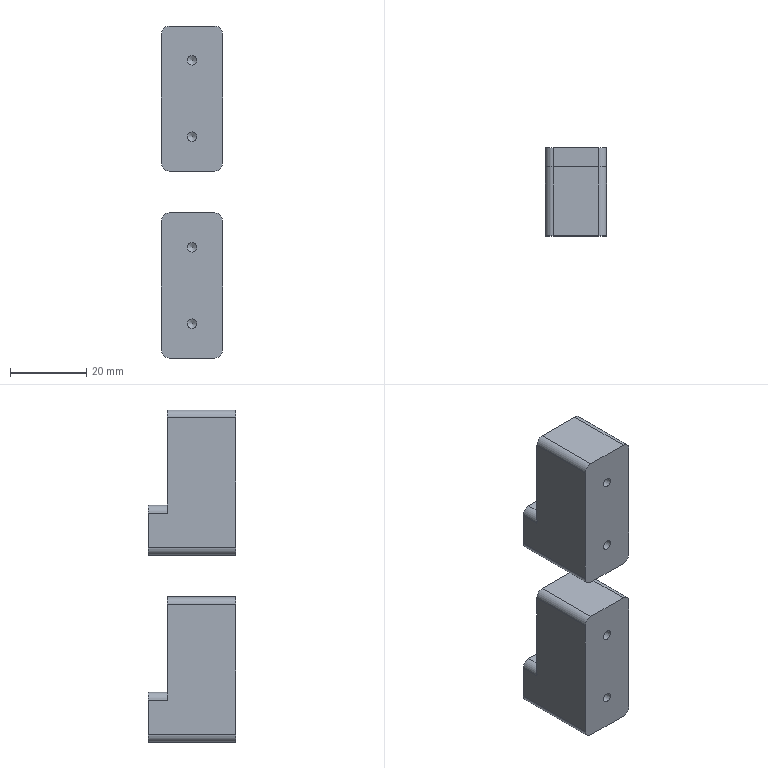Part | NX | 2 solids | 40 faces | box 16 x 23 x 87 mm | volume 23381 mm3 | cylinder 18 | plane 16 | cone 6 | commonest cylinder face diameters 4 x12 2.5 x4 3.3 x2
STEP:
#1=CARTESIAN_POINT('',(0.,18.,64.65));
#2=VERTEX_POINT('',#1);
#3=CARTESIAN_POINT('',(0.,18.,63.));
#4=DIRECTION('',(0.,1.,0.));
#5=DIRECTION('',(0.,0.,1.));
#6=AXIS2_PLACEMENT_3D('',#3,#4,#5);
#7=CIRCLE('',#6,1.65);
#8=EDGE_CURVE('',#2,#2,#7,.T.);
#9=ORIENTED_EDGE('',*,*,#8,.T.);
#10=EDGE_LOOP('',(#9));
#11=FACE_BOUND('',#10,.T.);
#12=CARTESIAN_POINT('',(0.,7.9,64.65));
#13=VERTEX_POINT('',#12);
#14=CARTESIAN_POINT('',(0.,7.9,63.));
#15=DIRECTION('',(0.,1.,0.));
#16=DIRECTION('',(0.,0.,1.));
#17=AXIS2_PLACEMENT_3D('',#14,#15,#16);
#18=CIRCLE('',#17,1.65);
#19=EDGE_CURVE('',#13,#13,#18,.T.);
#20=ORIENTED_EDGE('',*,*,#19,.F.);
#21=EDGE_LOOP('',(#20));
#22=FACE_BOUND('',#21,.T.);
#23=CARTESIAN_POINT('',(0.,18.,63.));
#24=DIRECTION('',(0.,1.,0.));
#25=DIRECTION('',(0.,0.,1.));
#26=AXIS2_PLACEMENT_3D('',#23,#24,#25);
#27=CYLINDRICAL_SURFACE('',#26,1.65);
#28=ADVANCED_FACE('',(#11,#22),#27,.F.);
#29=CARTESIAN_POINT('',(0.,6.909,63.));
#30=VERTEX_POINT('',#29);
#31=VERTEX_LOOP('',#30);
#32=FACE_BOUND('',#31,.T.);
#33=ORIENTED_EDGE('',*,*,#19,.T.);
#34=EDGE_LOOP('',(#33));
#35=FACE_BOUND('',#34,.T.);
#36=CARTESIAN_POINT('',(0.,7.9,63.));
#37=DIRECTION('',(0.,1.,0.));
#38=DIRECTION('',(0.,0.,1.));
#39=AXIS2_PLACEMENT_3D('',#36,#37,#38);
#40=CONICAL_SURFACE('',#39,1.65,1.03);
#41=ADVANCED_FACE('',(#32,#35),#40,.F.);
#42=CARTESIAN_POINT('',(6.,18.,68.));
#43=VERTEX_POINT('',#42);
#44=CARTESIAN_POINT('',(8.,18.,66.));
#45=VERTEX_POINT('',#44);
#46=CARTESIAN_POINT('',(6.,18.,66.));
#47=DIRECTION('',(0.,1.,0.));
#48=DIRECTION('',(0.,0.,-1.));
#49=AXIS2_PLACEMENT_3D('',#46,#47,#48);
#50=CIRCLE('',#49,2.);
#51=EDGE_CURVE('',#43,#45,#50,.T.);
#52=ORIENTED_EDGE('',*,*,#51,.F.);
#53=CARTESIAN_POINT('',(6.,0.,68.));
#54=VERTEX_POINT('',#53);
#55=CARTESIAN_POINT('',(6.,23.,68.));
#56=DIRECTION('',(0.,1.,0.));
#57=VECTOR('',#56,1000.);
#58=LINE('',#55,#57);
#59=EDGE_CURVE('',#54,#43,#58,.T.);
#60=ORIENTED_EDGE('',*,*,#59,.F.);
#61=CARTESIAN_POINT('',(8.,0.,66.));
#62=VERTEX_POINT('',#61);
#63=CARTESIAN_POINT('',(6.,0.,66.));
#64=DIRECTION('',(0.,-1.,0.));
#65=DIRECTION('',(0.,0.,-1.));
#66=AXIS2_PLACEMENT_3D('',#63,#64,#65);
#67=CIRCLE('',#66,2.);
#68=EDGE_CURVE('',#62,#54,#67,.T.);
#69=ORIENTED_EDGE('',*,*,#68,.F.);
#70=CARTESIAN_POINT('',(8.,23.,66.));
#71=DIRECTION('',(0.,-1.,0.));
#72=VECTOR('',#71,1000.);
#73=LINE('',#70,#72);
#74=EDGE_CURVE('',#45,#62,#73,.T.);
#75=ORIENTED_EDGE('',*,*,#74,.F.);
#76=EDGE_LOOP('',(#52,#60,#69,#75));
#77=FACE_BOUND('',#76,.T.);
#78=CARTESIAN_POINT('',(6.,23.,66.));
#79=DIRECTION('',(0.,-1.,0.));
#80=DIRECTION('',(0.,0.,-1.));
#81=AXIS2_PLACEMENT_3D('',#78,#79,#80);
#82=CYLINDRICAL_SURFACE('',#81,2.);
#83=ADVANCED_FACE('',(#77),#82,.T.);
#84=CARTESIAN_POINT('',(8.,23.,32.));
#85=VERTEX_POINT('',#84);
#86=CARTESIAN_POINT('',(6.,23.,30.));
#87=VERTEX_POINT('',#86);
#88=CARTESIAN_POINT('',(6.,23.,32.));
#89=DIRECTION('',(0.,1.,0.));
#90=DIRECTION('',(0.,0.,-1.));
#91=AXIS2_PLACEMENT_3D('',#88,#89,#90);
#92=CIRCLE('',#91,2.);
#93=EDGE_CURVE('',#85,#87,#92,.T.);
#94=ORIENTED_EDGE('',*,*,#93,.F.);
#95=CARTESIAN_POINT('',(8.,0.,32.));
#96=VERTEX_POINT('',#95);
#97=CARTESIAN_POINT('',(8.,23.,32.));
#98=DIRECTION('',(0.,1.,0.));
#99=VECTOR('',#98,1000.);
#100=LINE('',#97,#99);
#101=EDGE_CURVE('',#96,#85,#100,.T.);
#102=ORIENTED_EDGE('',*,*,#101,.F.);
#103=CARTESIAN_POINT('',(6.,0.,30.));
#104=VERTEX_POINT('',#103);
#105=CARTESIAN_POINT('',(6.,0.,32.));
#106=DIRECTION('',(0.,-1.,0.));
#107=DIRECTION('',(0.,0.,-1.));
#108=AXIS2_PLACEMENT_3D('',#105,#106,#107);
#109=CIRCLE('',#108,2.);
#110=EDGE_CURVE('',#104,#96,#109,.T.);
#111=ORIENTED_EDGE('',*,*,#110,.F.);
#112=CARTESIAN_POINT('',(6.,23.,30.));
#113=DIRECTION('',(0.,-1.,0.));
#114=VECTOR('',#113,1000.);
#115=LINE('',#112,#114);
#116=EDGE_CURVE('',#87,#104,#115,.T.);
#117=ORIENTED_EDGE('',*,*,#116,.F.);
#118=EDGE_LOOP('',(#94,#102,#111,#117));
#119=FACE_BOUND('',#118,.T.);
#120=CARTESIAN_POINT('',(6.,23.,32.));
#121=DIRECTION('',(0.,-1.,0.));
#122=DIRECTION('',(0.,0.,-1.));
#123=AXIS2_PLACEMENT_3D('',#120,#121,#122);
#124=CYLINDRICAL_SURFACE('',#123,2.);
#125=ADVANCED_FACE('',(#119),#124,.T.);
#126=CARTESIAN_POINT('',(-6.,23.,30.));
#127=VERTEX_POINT('',#126);
#128=CARTESIAN_POINT('',(-8.,23.,32.));
#129=VERTEX_POINT('',#128);
#130=CARTESIAN_POINT('',(-6.,23.,32.));
#131=DIRECTION('',(0.,1.,0.));
#132=DIRECTION('',(0.,0.,-1.));
#133=AXIS2_PLACEMENT_3D('',#130,#131,#132);
#134=CIRCLE('',#133,2.);
#135=EDGE_CURVE('',#127,#129,#134,.T.);
#136=ORIENTED_EDGE('',*,*,#135,.F.);
#137=CARTESIAN_POINT('',(-6.,0.,30.));
#138=VERTEX_POINT('',#137);
#139=CARTESIAN_POINT('',(-6.,23.,30.));
#140=DIRECTION('',(0.,1.,0.));
#141=VECTOR('',#140,1000.);
#142=LINE('',#139,#141);
#143=EDGE_CURVE('',#138,#127,#142,.T.);
#144=ORIENTED_EDGE('',*,*,#143,.F.);
#145=CARTESIAN_POINT('',(-8.,0.,32.));
#146=VERTEX_POINT('',#145);
#147=CARTESIAN_POINT('',(-6.,0.,32.));
#148=DIRECTION('',(0.,-1.,0.));
#149=DIRECTION('',(0.,0.,-1.));
#150=AXIS2_PLACEMENT_3D('',#147,#148,#149);
#151=CIRCLE('',#150,2.);
#152=EDGE_CURVE('',#146,#138,#151,.T.);
#153=ORIENTED_EDGE('',*,*,#152,.F.);
#154=CARTESIAN_POINT('',(-8.,23.,32.));
#155=DIRECTION('',(0.,-1.,0.));
#156=VECTOR('',#155,1000.);
#157=LINE('',#154,#156);
#158=EDGE_CURVE('',#129,#146,#157,.T.);
#159=ORIENTED_EDGE('',*,*,#158,.F.);
#160=EDGE_LOOP('',(#136,#144,#153,#159));
#161=FACE_BOUND('',#160,.T.);
#162=CARTESIAN_POINT('',(-6.,23.,32.));
#163=DIRECTION('',(0.,-1.,0.));
#164=DIRECTION('',(0.,0.,-1.));
#165=AXIS2_PLACEMENT_3D('',#162,#163,#164);
#166=CYLINDRICAL_SURFACE('',#165,2.);
#167=ADVANCED_FACE('',(#161),#166,.T.);
#168=CARTESIAN_POINT('',(-8.,18.,66.));
#169=VERTEX_POINT('',#168);
#170=CARTESIAN_POINT('',(-6.,18.,68.));
#171=VERTEX_POINT('',#170);
#172=CARTESIAN_POINT('',(-6.,18.,66.));
#173=DIRECTION('',(0.,1.,0.));
#174=DIRECTION('',(0.,0.,-1.));
#175=AXIS2_PLACEMENT_3D('',#172,#173,#174);
#176=CIRCLE('',#175,2.);
#177=EDGE_CURVE('',#169,#171,#176,.T.);
#178=ORIENTED_EDGE('',*,*,#177,.F.);
#179=CARTESIAN_POINT('',(-8.,0.,66.));
#180=VERTEX_POINT('',#179);
#181=CARTESIAN_POINT('',(-8.,23.,66.));
#182=DIRECTION('',(0.,1.,0.));
#183=VECTOR('',#182,1000.);
#184=LINE('',#181,#183);
#185=EDGE_CURVE('',#180,#169,#184,.T.);
#186=ORIENTED_EDGE('',*,*,#185,.F.);
#187=CARTESIAN_POINT('',(-6.,0.,68.));
#188=VERTEX_POINT('',#187);
#189=CARTESIAN_POINT('',(-6.,0.,66.));
#190=DIRECTION('',(0.,-1.,0.));
#191=DIRECTION('',(0.,0.,-1.));
#192=AXIS2_PLACEMENT_3D('',#189,#190,#191);
#193=CIRCLE('',#192,2.);
#194=EDGE_CURVE('',#188,#180,#193,.T.);
#195=ORIENTED_EDGE('',*,*,#194,.F.);
#196=CARTESIAN_POINT('',(-6.,23.,68.));
#197=DIRECTION('',(0.,-1.,0.));
#198=VECTOR('',#197,1000.);
#199=LINE('',#196,#198);
#200=EDGE_CURVE('',#171,#188,#199,.T.);
#201=ORIENTED_EDGE('',*,*,#200,.F.);
#202=EDGE_LOOP('',(#178,#186,#195,#201));
#203=FACE_BOUND('',#202,.T.);
#204=CARTESIAN_POINT('',(-6.,23.,66.));
#205=DIRECTION('',(0.,-1.,0.));
#206=DIRECTION('',(0.,0.,-1.));
#207=AXIS2_PLACEMENT_3D('',#204,#205,#206);
#208=CYLINDRICAL_SURFACE('',#207,2.);
#209=ADVANCED_FACE('',(#203),#208,.T.);
#210=CARTESIAN_POINT('',(-6.,18.,43.));
#211=VERTEX_POINT('',#210);
#212=CARTESIAN_POINT('',(-8.,18.,41.));
#213=VERTEX_POINT('',#212);
#214=CARTESIAN_POINT('',(-6.,18.,41.));
#215=DIRECTION('',(0.,-1.,0.));
#216=DIRECTION('',(0.,0.,-1.));
#217=AXIS2_PLACEMENT_3D('',#214,#215,#216);
#218=CIRCLE('',#217,2.);
#219=EDGE_CURVE('',#211,#213,#218,.T.);
#220=ORIENTED_EDGE('',*,*,#219,.F.);
#221=CARTESIAN_POINT('',(-6.,23.,43.));
#222=VERTEX_POINT('',#221);
#223=CARTESIAN_POINT('',(-6.,18.,43.));
#224=DIRECTION('',(0.,-1.,0.));
#225=VECTOR('',#224,1000.);
#226=LINE('',#223,#225);
#227=EDGE_CURVE('',#222,#211,#226,.T.);
#228=ORIENTED_EDGE('',*,*,#227,.F.);
#229=CARTESIAN_POINT('',(-8.,23.,41.));
#230=VERTEX_POINT('',#229);
#231=CARTESIAN_POINT('',(-6.,23.,41.));
#232=DIRECTION('',(0.,1.,0.));
#233=DIRECTION('',(0.,0.,-1.));
#234=AXIS2_PLACEMENT_3D('',#231,#232,#233);
#235=CIRCLE('',#234,2.);
#236=EDGE_CURVE('',#230,#222,#235,.T.);
#237=ORIENTED_EDGE('',*,*,#236,.F.);
#238=CARTESIAN_POINT('',(-8.,23.,41.));
#239=DIRECTION('',(0.,1.,0.));
#240=VECTOR('',#239,1000.);
#241=LINE('',#238,#240);
#242=EDGE_CURVE('',#213,#230,#241,.T.);
#243=ORIENTED_EDGE('',*,*,#242,.F.);
#244=EDGE_LOOP('',(#220,#228,#237,#243));
#245=FACE_BOUND('',#244,.T.);
#246=CARTESIAN_POINT('',(-6.,23.,41.));
#247=DIRECTION('',(0.,-1.,0.));
#248=DIRECTION('',(0.,0.,-1.));
#249=AXIS2_PLACEMENT_3D('',#246,#247,#248);
#250=CYLINDRICAL_SURFACE('',#249,2.);
#251=ADVANCED_FACE('',(#245),#250,.T.);
#252=CARTESIAN_POINT('',(8.,18.,41.));
#253=VERTEX_POINT('',#252);
#254=CARTESIAN_POINT('',(6.,18.,43.));
#255=VERTEX_POINT('',#254);
#256=CARTESIAN_POINT('',(6.,18.,41.));
#257=DIRECTION('',(0.,-1.,0.));
#258=DIRECTION('',(0.,0.,-1.));
#259=AXIS2_PLACEMENT_3D('',#256,#257,#258);
#260=CIRCLE('',#259,2.);
#261=EDGE_CURVE('',#253,#255,#260,.T.);
#262=ORIENTED_EDGE('',*,*,#261,.F.);
#263=CARTESIAN_POINT('',(8.,23.,41.));
#264=VERTEX_POINT('',#263);
#265=CARTESIAN_POINT('',(8.,18.,41.));
#266=DIRECTION('',(0.,-1.,0.));
#267=VECTOR('',#266,1000.);
#268=LINE('',#265,#267);
#269=EDGE_CURVE('',#264,#253,#268,.T.);
#270=ORIENTED_EDGE('',*,*,#269,.F.);
#271=CARTESIAN_POINT('',(6.,23.,43.));
#272=VERTEX_POINT('',#271);
#273=CARTESIAN_POINT('',(6.,23.,41.));
#274=DIRECTION('',(0.,1.,0.));
#275=DIRECTION('',(0.,0.,-1.));
#276=AXIS2_PLACEMENT_3D('',#273,#274,#275);
#277=CIRCLE('',#276,2.);
#278=EDGE_CURVE('',#272,#264,#277,.T.);
#279=ORIENTED_EDGE('',*,*,#278,.F.);
#280=CARTESIAN_POINT('',(6.,23.,43.));
#281=DIRECTION('',(0.,1.,0.));
#282=VECTOR('',#281,1000.);
#283=LINE('',#280,#282);
#284=EDGE_CURVE('',#255,#272,#283,.T.);
#285=ORIENTED_EDGE('',*,*,#284,.F.);
#286=EDGE_LOOP('',(#262,#270,#279,#285));
#287=FACE_BOUND('',#286,.T.);
#288=CARTESIAN_POINT('',(6.,18.,41.));
#289=DIRECTION('',(0.,-1.,0.));
#290=DIRECTION('',(0.,0.,-1.));
#291=AXIS2_PLACEMENT_3D('',#288,#289,#290);
#292=CYLINDRICAL_SURFACE('',#291,2.);
#293=ADVANCED_FACE('',(#287),#292,.T.);
#294=CARTESIAN_POINT('',(-8.,18.,43.));
#295=DIRECTION('',(0.,0.,-1.));
#296=VECTOR('',#295,1000.);
#297=LINE('',#294,#296);
#298=EDGE_CURVE('',#169,#213,#297,.T.);
#299=ORIENTED_EDGE('',*,*,#298,.F.);
#300=ORIENTED_EDGE('',*,*,#177,.T.);
#301=CARTESIAN_POINT('',(8.,18.,68.));
#302=DIRECTION('',(-1.,0.,0.));
#303=VECTOR('',#302,1000.);
#304=LINE('',#301,#303);
#305=EDGE_CURVE('',#43,#171,#304,.T.);
#306=ORIENTED_EDGE('',*,*,#305,.F.);
#307=ORIENTED_EDGE('',*,*,#51,.T.);
#308=CARTESIAN_POINT('',(8.,18.,43.));
#309=DIRECTION('',(0.,0.,1.));
#310=VECTOR('',#309,1000.);
#311=LINE('',#308,#310);
#312=EDGE_CURVE('',#253,#45,#311,.T.);
#313=ORIENTED_EDGE('',*,*,#312,.F.);
#314=ORIENTED_EDGE('',*,*,#261,.T.);
#315=CARTESIAN_POINT('',(8.,18.,43.));
#316=DIRECTION('',(1.,0.,0.));
#317=VECTOR('',#316,1000.);
#318=LINE('',#315,#317);
#319=EDGE_CURVE('',#211,#255,#318,.T.);
#320=ORIENTED_EDGE('',*,*,#319,.F.);
#321=ORIENTED_EDGE('',*,*,#219,.T.);
#322=EDGE_LOOP('',(#299,#300,#306,#307,#313,#314,#320,#321));
#323=FACE_BOUND('',#322,.T.);
#324=ORIENTED_EDGE('',*,*,#8,.F.);
#325=EDGE_LOOP('',(#324));
#326=FACE_BOUND('',#325,.T.);
#327=CARTESIAN_POINT('',(0.,18.,49.));
#328=DIRECTION('',(0.,-1.,0.));
#329=DIRECTION('',(0.,0.,-1.));
#330=AXIS2_PLACEMENT_3D('',#327,#328,#329);
#331=PLANE('',#330);
#332=ADVANCED_FACE('',(#323,#326),#331,.F.);
#333=ORIENTED_EDGE('',*,*,#319,.T.);
#334=ORIENTED_EDGE('',*,*,#284,.T.);
#335=CARTESIAN_POINT('',(8.,23.,43.));
#336=DIRECTION('',(1.,0.,0.));
#337=VECTOR('',#336,1000.);
#338=LINE('',#335,#337);
#339=EDGE_CURVE('',#222,#272,#338,.T.);
#340=ORIENTED_EDGE('',*,*,#339,.F.);
#341=ORIENTED_EDGE('',*,*,#227,.T.);
#342=EDGE_LOOP('',(#333,#334,#340,#341));
#343=FACE_BOUND('',#342,.T.);
#344=CARTESIAN_POINT('',(8.,18.,43.));
#345=DIRECTION('',(0.,0.,1.));
#346=DIRECTION('',(1.,0.,0.));
#347=AXIS2_PLACEMENT_3D('',#344,#345,#346);
#348=PLANE('',#347);
#349=ADVANCED_FACE('',(#343),#348,.T.);
#350=CARTESIAN_POINT('',(0.,0.,37.75));
#351=VERTEX_POINT('',#350);
#352=CARTESIAN_POINT('',(0.,0.,39.));
#353=DIRECTION('',(0.,-1.,0.));
#354=DIRECTION('',(0.,0.,-1.));
#355=AXIS2_PLACEMENT_3D('',#352,#353,#354);
#356=CIRCLE('',#355,1.25);
#357=EDGE_CURVE('',#351,#351,#356,.T.);
#358=ORIENTED_EDGE('',*,*,#357,.T.);
#359=EDGE_LOOP('',(#358));
#360=FACE_BOUND('',#359,.T.);
#361=CARTESIAN_POINT('',(0.,12.5,37.75));
#362=VERTEX_POINT('',#361);
#363=CARTESIAN_POINT('',(0.,12.5,39.));
#364=DIRECTION('',(0.,-1.,0.));
#365=DIRECTION('',(0.,0.,-1.));
#366=AXIS2_PLACEMENT_3D('',#363,#364,#365);
#367=CIRCLE('',#366,1.25);
#368=EDGE_CURVE('',#362,#362,#367,.T.);
#369=ORIENTED_EDGE('',*,*,#368,.F.);
#370=EDGE_LOOP('',(#369));
#371=FACE_BOUND('',#370,.T.);
#372=CARTESIAN_POINT('',(0.,0.,39.));
#373=DIRECTION('',(0.,-1.,0.));
#374=DIRECTION('',(0.,0.,-1.));
#375=AXIS2_PLACEMENT_3D('',#372,#373,#374);
#376=CYLINDRICAL_SURFACE('',#375,1.25);
#377=ADVANCED_FACE('',(#360,#371),#376,.F.);
#378=CARTESIAN_POINT('',(0.,13.251,39.));
#379=VERTEX_POINT('',#378);
#380=VERTEX_LOOP('',#379);
#381=FACE_BOUND('',#380,.T.);
#382=ORIENTED_EDGE('',*,*,#368,.T.);
#383=EDGE_LOOP('',(#382));
#384=FACE_BOUND('',#383,.T.);
#385=CARTESIAN_POINT('',(0.,12.5,39.));
#386=DIRECTION('',(0.,-1.,0.));
#387=DIRECTION('',(0.,0.,-1.));
#388=AXIS2_PLACEMENT_3D('',#385,#386,#387);
#389=CONICAL_SURFACE('',#388,1.25,1.03);
#390=ADVANCED_FACE('',(#381,#384),#389,.F.);
#391=CARTESIAN_POINT('',(0.,0.,57.75));
#392=VERTEX_POINT('',#391);
#393=CARTESIAN_POINT('',(0.,0.,59.));
#394=DIRECTION('',(0.,-1.,0.));
#395=DIRECTION('',(0.,0.,-1.));
#396=AXIS2_PLACEMENT_3D('',#393,#394,#395);
#397=CIRCLE('',#396,1.25);
#398=EDGE_CURVE('',#392,#392,#397,.T.);
#399=ORIENTED_EDGE('',*,*,#398,.T.);
#400=EDGE_LOOP('',(#399));
#401=FACE_BOUND('',#400,.T.);
#402=CARTESIAN_POINT('',(0.,12.5,57.75));
#403=VERTEX_POINT('',#402);
#404=CARTESIAN_POINT('',(0.,12.5,59.));
#405=DIRECTION('',(0.,-1.,0.));
#406=DIRECTION('',(0.,0.,-1.));
#407=AXIS2_PLACEMENT_3D('',#404,#405,#406);
#408=CIRCLE('',#407,1.25);
#409=EDGE_CURVE('',#403,#403,#408,.T.);
#410=ORIENTED_EDGE('',*,*,#409,.F.);
#411=EDGE_LOOP('',(#410));
#412=FACE_BOUND('',#411,.T.);
#413=CARTESIAN_POINT('',(0.,0.,59.));
#414=DIRECTION('',(0.,-1.,0.));
#415=DIRECTION('',(0.,0.,-1.));
#416=AXIS2_PLACEMENT_3D('',#413,#414,#415);
#417=CYLINDRICAL_SURFACE('',#416,1.25);
#418=ADVANCED_FACE('',(#401,#412),#417,.F.);
#419=CARTESIAN_POINT('',(0.,13.251,59.));
#420=VERTEX_POINT('',#419);
#421=VERTEX_LOOP('',#420);
#422=FACE_BOUND('',#421,.T.);
#423=ORIENTED_EDGE('',*,*,#409,.T.);
#424=EDGE_LOOP('',(#423));
#425=FACE_BOUND('',#424,.T.);
#426=CARTESIAN_POINT('',(0.,12.5,59.));
#427=DIRECTION('',(0.,-1.,0.));
#428=DIRECTION('',(0.,0.,-1.));
#429=AXIS2_PLACEMENT_3D('',#426,#427,#428);
#430=CONICAL_SURFACE('',#429,1.25,1.03);
#431=ADVANCED_FACE('',(#422,#425),#430,.F.);
#432=CARTESIAN_POINT('',(-8.,0.,68.));
#433=DIRECTION('',(1.,0.,0.));
#434=VECTOR('',#433,1000.);
#435=LINE('',#432,#434);
#436=EDGE_CURVE('',#188,#54,#435,.T.);
#437=ORIENTED_EDGE('',*,*,#436,.F.);
#438=ORIENTED_EDGE('',*,*,#194,.T.);
#439=CARTESIAN_POINT('',(-8.,0.,68.));
#440=DIRECTION('',(0.,0.,1.));
#441=VECTOR('',#440,1000.);
#442=LINE('',#439,#441);
#443=EDGE_CURVE('',#146,#180,#442,.T.);
#444=ORIENTED_EDGE('',*,*,#443,.F.);
#445=ORIENTED_EDGE('',*,*,#152,.T.);
#446=CARTESIAN_POINT('',(-8.,0.,30.));
#447=DIRECTION('',(-1.,0.,0.));
#448=VECTOR('',#447,1000.);
#449=LINE('',#446,#448);
#450=EDGE_CURVE('',#104,#138,#449,.T.);
#451=ORIENTED_EDGE('',*,*,#450,.F.);
#452=ORIENTED_EDGE('',*,*,#110,.T.);
#453=CARTESIAN_POINT('',(8.,0.,68.));
#454=DIRECTION('',(0.,0.,-1.));
#455=VECTOR('',#454,1000.);
#456=LINE('',#453,#455);
#457=EDGE_CURVE('',#62,#96,#456,.T.);
#458=ORIENTED_EDGE('',*,*,#457,.F.);
#459=ORIENTED_EDGE('',*,*,#68,.T.);
#460=EDGE_LOOP('',(#437,#438,#444,#445,#451,#452,#458,#459));
#461=FACE_BOUND('',#460,.T.);
#462=ORIENTED_EDGE('',*,*,#398,.F.);
#463=EDGE_LOOP('',(#462));
#464=FACE_BOUND('',#463,.T.);
#465=ORIENTED_EDGE('',*,*,#357,.F.);
#466=EDGE_LOOP('',(#465));
#467=FACE_BOUND('',#466,.T.);
#468=CARTESIAN_POINT('',(0.,0.,49.));
#469=DIRECTION('',(0.,-1.,0.));
#470=DIRECTION('',(0.,0.,-1.));
#471=AXIS2_PLACEMENT_3D('',#468,#469,#470);
#472=PLANE('',#471);
#473=ADVANCED_FACE('',(#461,#464,#467),#472,.T.);
#474=ORIENTED_EDGE('',*,*,#305,.T.);
#475=ORIENTED_EDGE('',*,*,#200,.T.);
#476=ORIENTED_EDGE('',*,*,#436,.T.);
#477=ORIENTED_EDGE('',*,*,#59,.T.);
#478=EDGE_LOOP('',(#474,#475,#476,#477));
#479=FACE_BOUND('',#478,.T.);
#480=CARTESIAN_POINT('',(-8.,23.,68.));
#481=DIRECTION('',(0.,0.,-1.));
#482=DIRECTION('',(-1.,0.,0.));
#483=AXIS2_PLACEMENT_3D('',#480,#481,#482);
#484=PLANE('',#483);
#485=ADVANCED_FACE('',(#479),#484,.F.);
#486=ORIENTED_EDGE('',*,*,#450,.T.);
#487=ORIENTED_EDGE('',*,*,#143,.T.);
#488=CARTESIAN_POINT('',(-8.,23.,30.));
#489=DIRECTION('',(-1.,0.,0.));
#490=VECTOR('',#489,1000.);
#491=LINE('',#488,#490);
#492=EDGE_CURVE('',#87,#127,#491,.T.);
#493=ORIENTED_EDGE('',*,*,#492,.F.);
#494=ORIENTED_EDGE('',*,*,#116,.T.);
#495=EDGE_LOOP('',(#486,#487,#493,#494));
#496=FACE_BOUND('',#495,.T.);
#497=CARTESIAN_POINT('',(-8.,23.,30.));
#498=DIRECTION('',(0.,0.,1.));
#499=DIRECTION('',(1.,0.,0.));
#500=AXIS2_PLACEMENT_3D('',#497,#498,#499);
#501=PLANE('',#500);
#502=ADVANCED_FACE('',(#496),#501,.F.);
#503=ORIENTED_EDGE('',*,*,#339,.T.);
#504=ORIENTED_EDGE('',*,*,#278,.T.);
#505=CARTESIAN_POINT('',(8.,23.,68.));
#506=DIRECTION('',(0.,0.,-1.));
#507=VECTOR('',#506,1000.);
#508=LINE('',#505,#507);
#509=EDGE_CURVE('',#264,#85,#508,.T.);
#510=ORIENTED_EDGE('',*,*,#509,.T.);
#511=ORIENTED_EDGE('',*,*,#93,.T.);
#512=ORIENTED_EDGE('',*,*,#492,.T.);
#513=ORIENTED_EDGE('',*,*,#135,.T.);
#514=CARTESIAN_POINT('',(-8.,23.,68.));
#515=DIRECTION('',(0.,0.,1.));
#516=VECTOR('',#515,1000.);
#517=LINE('',#514,#516);
#518=EDGE_CURVE('',#129,#230,#517,.T.);
#519=ORIENTED_EDGE('',*,*,#518,.T.);
#520=ORIENTED_EDGE('',*,*,#236,.T.);
#521=EDGE_LOOP('',(#503,#504,#510,#511,#512,#513,#519,#520));
#522=FACE_BOUND('',#521,.T.);
#523=CARTESIAN_POINT('',(0.,23.,49.));
#524=DIRECTION('',(0.,-1.,0.));
#525=DIRECTION('',(0.,0.,-1.));
#526=AXIS2_PLACEMENT_3D('',#523,#524,#525);
#527=PLANE('',#526);
#528=ADVANCED_FACE('',(#522),#527,.F.);
#529=ORIENTED_EDGE('',*,*,#298,.T.);
#530=ORIENTED_EDGE('',*,*,#242,.T.);
#531=ORIENTED_EDGE('',*,*,#518,.F.);
#532=ORIENTED_EDGE('',*,*,#158,.T.);
#533=ORIENTED_EDGE('',*,*,#443,.T.);
#534=ORIENTED_EDGE('',*,*,#185,.T.);
#535=EDGE_LOOP('',(#529,#530,#531,#532,#533,#534));
#536=FACE_BOUND('',#535,.T.);
#537=CARTESIAN_POINT('',(-8.,23.,68.));
#538=DIRECTION('',(1.,0.,0.));
#539=DIRECTION('',(0.,0.,-1.));
#540=AXIS2_PLACEMENT_3D('',#537,#538,#539);
#541=PLANE('',#540);
#542=ADVANCED_FACE('',(#536),#541,.F.);
#543=ORIENTED_EDGE('',*,*,#509,.F.);
#544=ORIENTED_EDGE('',*,*,#269,.T.);
#545=ORIENTED_EDGE('',*,*,#312,.T.);
#546=ORIENTED_EDGE('',*,*,#74,.T.);
#547=ORIENTED_EDGE('',*,*,#457,.T.);
#548=ORIENTED_EDGE('',*,*,#101,.T.);
#549=EDGE_LOOP('',(#543,#544,#545,#546,#547,#548));
#550=FACE_BOUND('',#549,.T.);
#551=CARTESIAN_POINT('',(8.,23.,68.));
#552=DIRECTION('',(-1.,0.,0.));
#553=DIRECTION('',(0.,0.,1.));
#554=AXIS2_PLACEMENT_3D('',#551,#552,#553);
#555=PLANE('',#554);
#556=ADVANCED_FACE('',(#550),#555,.F.);
#557=CLOSED_SHELL('',(#28,#41,#83,#125,#167,#209,#251,#293,#332,#349,#377,#390,#418,#431,#473,#485,#502,#528,#542,#556));
#558=MANIFOLD_SOLID_BREP('',#557);
#559=CARTESIAN_POINT('',(0.,18.,15.65));
#560=VERTEX_POINT('',#559);
#561=CARTESIAN_POINT('',(0.,18.,14.));
#562=DIRECTION('',(0.,1.,0.));
#563=DIRECTION('',(0.,0.,1.));
#564=AXIS2_PLACEMENT_3D('',#561,#562,#563);
#565=CIRCLE('',#564,1.65);
#566=EDGE_CURVE('',#560,#560,#565,.T.);
#567=ORIENTED_EDGE('',*,*,#566,.T.);
#568=EDGE_LOOP('',(#567));
#569=FACE_BOUND('',#568,.T.);
#570=CARTESIAN_POINT('',(0.,7.9,15.65));
#571=VERTEX_POINT('',#570);
#572=CARTESIAN_POINT('',(0.,7.9,14.));
#573=DIRECTION('',(0.,1.,0.));
#574=DIRECTION('',(0.,0.,1.));
#575=AXIS2_PLACEMENT_3D('',#572,#573,#574);
#576=CIRCLE('',#575,1.65);
#577=EDGE_CURVE('',#571,#571,#576,.T.);
#578=ORIENTED_EDGE('',*,*,#577,.F.);
#579=EDGE_LOOP('',(#578));
#580=FACE_BOUND('',#579,.T.);
#581=CARTESIAN_POINT('',(0.,18.,14.));
#582=DIRECTION('',(0.,1.,0.));
#583=DIRECTION('',(0.,0.,1.));
#584=AXIS2_PLACEMENT_3D('',#581,#582,#583);
#585=CYLINDRICAL_SURFACE('',#584,1.65);
#586=ADVANCED_FACE('',(#569,#580),#585,.F.);
#587=CARTESIAN_POINT('',(0.,6.909,14.));
#588=VERTEX_POINT('',#587);
#589=VERTEX_LOOP('',#588);
#590=FACE_BOUND('',#589,.T.);
#591=ORIENTED_EDGE('',*,*,#577,.T.);
#592=EDGE_LOOP('',(#591));
#593=FACE_BOUND('',#592,.T.);
#594=CARTESIAN_POINT('',(0.,7.9,14.));
#595=DIRECTION('',(0.,1.,0.));
#596=DIRECTION('',(0.,0.,1.));
#597=AXIS2_PLACEMENT_3D('',#594,#595,#596);
#598=CONICAL_SURFACE('',#597,1.65,1.03);
#599=ADVANCED_FACE('',(#590,#593),#598,.F.);
#600=CARTESIAN_POINT('',(6.,18.,19.));
#601=VERTEX_POINT('',#600);
#602=CARTESIAN_POINT('',(8.,18.,17.));
#603=VERTEX_POINT('',#602);
#604=CARTESIAN_POINT('',(6.,18.,17.));
#605=DIRECTION('',(0.,1.,0.));
#606=DIRECTION('',(0.,0.,-1.));
#607=AXIS2_PLACEMENT_3D('',#604,#605,#606);
#608=CIRCLE('',#607,2.);
#609=EDGE_CURVE('',#601,#603,#608,.T.);
#610=ORIENTED_EDGE('',*,*,#609,.F.);
#611=CARTESIAN_POINT('',(6.,0.,19.));
#612=VERTEX_POINT('',#611);
#613=CARTESIAN_POINT('',(6.,23.,19.));
#614=DIRECTION('',(0.,1.,0.));
#615=VECTOR('',#614,1000.);
#616=LINE('',#613,#615);
#617=EDGE_CURVE('',#612,#601,#616,.T.);
#618=ORIENTED_EDGE('',*,*,#617,.F.);
#619=CARTESIAN_POINT('',(8.,0.,17.));
#620=VERTEX_POINT('',#619);
#621=CARTESIAN_POINT('',(6.,0.,17.));
#622=DIRECTION('',(0.,-1.,0.));
#623=DIRECTION('',(0.,0.,-1.));
#624=AXIS2_PLACEMENT_3D('',#621,#622,#623);
#625=CIRCLE('',#624,2.);
#626=EDGE_CURVE('',#620,#612,#625,.T.);
#627=ORIENTED_EDGE('',*,*,#626,.F.);
#628=CARTESIAN_POINT('',(8.,23.,17.));
#629=DIRECTION('',(0.,-1.,0.));
#630=VECTOR('',#629,1000.);
#631=LINE('',#628,#630);
#632=EDGE_CURVE('',#603,#620,#631,.T.);
#633=ORIENTED_EDGE('',*,*,#632,.F.);
#634=EDGE_LOOP('',(#610,#618,#627,#633));
#635=FACE_BOUND('',#634,.T.);
#636=CARTESIAN_POINT('',(6.,23.,17.));
#637=DIRECTION('',(0.,-1.,0.));
#638=DIRECTION('',(0.,0.,-1.));
#639=AXIS2_PLACEMENT_3D('',#636,#637,#638);
#640=CYLINDRICAL_SURFACE('',#639,2.);
#641=ADVANCED_FACE('',(#635),#640,.T.);
#642=CARTESIAN_POINT('',(8.,23.,-17.));
#643=VERTEX_POINT('',#642);
#644=CARTESIAN_POINT('',(6.,23.,-19.));
#645=VERTEX_POINT('',#644);
#646=CARTESIAN_POINT('',(6.,23.,-17.));
#647=DIRECTION('',(0.,1.,0.));
#648=DIRECTION('',(0.,0.,-1.));
#649=AXIS2_PLACEMENT_3D('',#646,#647,#648);
#650=CIRCLE('',#649,2.);
#651=EDGE_CURVE('',#643,#645,#650,.T.);
#652=ORIENTED_EDGE('',*,*,#651,.F.);
#653=CARTESIAN_POINT('',(8.,0.,-17.));
#654=VERTEX_POINT('',#653);
#655=CARTESIAN_POINT('',(8.,23.,-17.));
#656=DIRECTION('',(0.,1.,0.));
#657=VECTOR('',#656,1000.);
#658=LINE('',#655,#657);
#659=EDGE_CURVE('',#654,#643,#658,.T.);
#660=ORIENTED_EDGE('',*,*,#659,.F.);
#661=CARTESIAN_POINT('',(6.,0.,-19.));
#662=VERTEX_POINT('',#661);
#663=CARTESIAN_POINT('',(6.,0.,-17.));
#664=DIRECTION('',(0.,-1.,0.));
#665=DIRECTION('',(0.,0.,-1.));
#666=AXIS2_PLACEMENT_3D('',#663,#664,#665);
#667=CIRCLE('',#666,2.);
#668=EDGE_CURVE('',#662,#654,#667,.T.);
#669=ORIENTED_EDGE('',*,*,#668,.F.);
#670=CARTESIAN_POINT('',(6.,23.,-19.));
#671=DIRECTION('',(0.,-1.,0.));
#672=VECTOR('',#671,1000.);
#673=LINE('',#670,#672);
#674=EDGE_CURVE('',#645,#662,#673,.T.);
#675=ORIENTED_EDGE('',*,*,#674,.F.);
#676=EDGE_LOOP('',(#652,#660,#669,#675));
#677=FACE_BOUND('',#676,.T.);
#678=CARTESIAN_POINT('',(6.,23.,-17.));
#679=DIRECTION('',(0.,-1.,0.));
#680=DIRECTION('',(0.,0.,-1.));
#681=AXIS2_PLACEMENT_3D('',#678,#679,#680);
#682=CYLINDRICAL_SURFACE('',#681,2.);
#683=ADVANCED_FACE('',(#677),#682,.T.);
#684=CARTESIAN_POINT('',(-6.,23.,-19.));
#685=VERTEX_POINT('',#684);
#686=CARTESIAN_POINT('',(-8.,23.,-17.));
#687=VERTEX_POINT('',#686);
#688=CARTESIAN_POINT('',(-6.,23.,-17.));
#689=DIRECTION('',(0.,1.,0.));
#690=DIRECTION('',(0.,0.,-1.));
#691=AXIS2_PLACEMENT_3D('',#688,#689,#690);
#692=CIRCLE('',#691,2.);
#693=EDGE_CURVE('',#685,#687,#692,.T.);
#694=ORIENTED_EDGE('',*,*,#693,.F.);
#695=CARTESIAN_POINT('',(-6.,0.,-19.));
#696=VERTEX_POINT('',#695);
#697=CARTESIAN_POINT('',(-6.,23.,-19.));
#698=DIRECTION('',(0.,1.,0.));
#699=VECTOR('',#698,1000.);
#700=LINE('',#697,#699);
#701=EDGE_CURVE('',#696,#685,#700,.T.);
#702=ORIENTED_EDGE('',*,*,#701,.F.);
#703=CARTESIAN_POINT('',(-8.,0.,-17.));
#704=VERTEX_POINT('',#703);
#705=CARTESIAN_POINT('',(-6.,0.,-17.));
#706=DIRECTION('',(0.,-1.,0.));
#707=DIRECTION('',(0.,0.,-1.));
#708=AXIS2_PLACEMENT_3D('',#705,#706,#707);
#709=CIRCLE('',#708,2.);
#710=EDGE_CURVE('',#704,#696,#709,.T.);
#711=ORIENTED_EDGE('',*,*,#710,.F.);
#712=CARTESIAN_POINT('',(-8.,23.,-17.));
#713=DIRECTION('',(0.,-1.,0.));
#714=VECTOR('',#713,1000.);
#715=LINE('',#712,#714);
#716=EDGE_CURVE('',#687,#704,#715,.T.);
#717=ORIENTED_EDGE('',*,*,#716,.F.);
#718=EDGE_LOOP('',(#694,#702,#711,#717));
#719=FACE_BOUND('',#718,.T.);
#720=CARTESIAN_POINT('',(-6.,23.,-17.));
#721=DIRECTION('',(0.,-1.,0.));
#722=DIRECTION('',(0.,0.,-1.));
#723=AXIS2_PLACEMENT_3D('',#720,#721,#722);
#724=CYLINDRICAL_SURFACE('',#723,2.);
#725=ADVANCED_FACE('',(#719),#724,.T.);
#726=CARTESIAN_POINT('',(-8.,18.,17.));
#727=VERTEX_POINT('',#726);
#728=CARTESIAN_POINT('',(-6.,18.,19.));
#729=VERTEX_POINT('',#728);
#730=CARTESIAN_POINT('',(-6.,18.,17.));
#731=DIRECTION('',(0.,1.,0.));
#732=DIRECTION('',(0.,0.,-1.));
#733=AXIS2_PLACEMENT_3D('',#730,#731,#732);
#734=CIRCLE('',#733,2.);
#735=EDGE_CURVE('',#727,#729,#734,.T.);
#736=ORIENTED_EDGE('',*,*,#735,.F.);
#737=CARTESIAN_POINT('',(-8.,0.,17.));
#738=VERTEX_POINT('',#737);
#739=CARTESIAN_POINT('',(-8.,23.,17.));
#740=DIRECTION('',(0.,1.,0.));
#741=VECTOR('',#740,1000.);
#742=LINE('',#739,#741);
#743=EDGE_CURVE('',#738,#727,#742,.T.);
#744=ORIENTED_EDGE('',*,*,#743,.F.);
#745=CARTESIAN_POINT('',(-6.,0.,19.));
#746=VERTEX_POINT('',#745);
#747=CARTESIAN_POINT('',(-6.,0.,17.));
#748=DIRECTION('',(0.,-1.,0.));
#749=DIRECTION('',(0.,0.,-1.));
#750=AXIS2_PLACEMENT_3D('',#747,#748,#749);
#751=CIRCLE('',#750,2.);
#752=EDGE_CURVE('',#746,#738,#751,.T.);
#753=ORIENTED_EDGE('',*,*,#752,.F.);
#754=CARTESIAN_POINT('',(-6.,23.,19.));
#755=DIRECTION('',(0.,-1.,0.));
#756=VECTOR('',#755,1000.);
#757=LINE('',#754,#756);
#758=EDGE_CURVE('',#729,#746,#757,.T.);
#759=ORIENTED_EDGE('',*,*,#758,.F.);
#760=EDGE_LOOP('',(#736,#744,#753,#759));
#761=FACE_BOUND('',#760,.T.);
#762=CARTESIAN_POINT('',(-6.,23.,17.));
#763=DIRECTION('',(0.,-1.,0.));
#764=DIRECTION('',(0.,0.,-1.));
#765=AXIS2_PLACEMENT_3D('',#762,#763,#764);
#766=CYLINDRICAL_SURFACE('',#765,2.);
#767=ADVANCED_FACE('',(#761),#766,.T.);
#768=CARTESIAN_POINT('',(-6.,18.,-6.));
#769=VERTEX_POINT('',#768);
#770=CARTESIAN_POINT('',(-8.,18.,-8.));
#771=VERTEX_POINT('',#770);
#772=CARTESIAN_POINT('',(-6.,18.,-8.));
#773=DIRECTION('',(0.,-1.,0.));
#774=DIRECTION('',(0.,0.,-1.));
#775=AXIS2_PLACEMENT_3D('',#772,#773,#774);
#776=CIRCLE('',#775,2.);
#777=EDGE_CURVE('',#769,#771,#776,.T.);
#778=ORIENTED_EDGE('',*,*,#777,.F.);
#779=CARTESIAN_POINT('',(-6.,23.,-6.));
#780=VERTEX_POINT('',#779);
#781=CARTESIAN_POINT('',(-6.,18.,-6.));
#782=DIRECTION('',(0.,-1.,0.));
#783=VECTOR('',#782,1000.);
#784=LINE('',#781,#783);
#785=EDGE_CURVE('',#780,#769,#784,.T.);
#786=ORIENTED_EDGE('',*,*,#785,.F.);
#787=CARTESIAN_POINT('',(-8.,23.,-8.));
#788=VERTEX_POINT('',#787);
#789=CARTESIAN_POINT('',(-6.,23.,-8.));
#790=DIRECTION('',(0.,1.,0.));
#791=DIRECTION('',(0.,0.,-1.));
#792=AXIS2_PLACEMENT_3D('',#789,#790,#791);
#793=CIRCLE('',#792,2.);
#794=EDGE_CURVE('',#788,#780,#793,.T.);
#795=ORIENTED_EDGE('',*,*,#794,.F.);
#796=CARTESIAN_POINT('',(-8.,23.,-8.));
#797=DIRECTION('',(0.,1.,0.));
#798=VECTOR('',#797,1000.);
#799=LINE('',#796,#798);
#800=EDGE_CURVE('',#771,#788,#799,.T.);
#801=ORIENTED_EDGE('',*,*,#800,.F.);
#802=EDGE_LOOP('',(#778,#786,#795,#801));
#803=FACE_BOUND('',#802,.T.);
#804=CARTESIAN_POINT('',(-6.,23.,-8.));
#805=DIRECTION('',(0.,-1.,0.));
#806=DIRECTION('',(0.,0.,-1.));
#807=AXIS2_PLACEMENT_3D('',#804,#805,#806);
#808=CYLINDRICAL_SURFACE('',#807,2.);
#809=ADVANCED_FACE('',(#803),#808,.T.);
#810=CARTESIAN_POINT('',(8.,18.,-8.));
#811=VERTEX_POINT('',#810);
#812=CARTESIAN_POINT('',(6.,18.,-6.));
#813=VERTEX_POINT('',#812);
#814=CARTESIAN_POINT('',(6.,18.,-8.));
#815=DIRECTION('',(0.,-1.,0.));
#816=DIRECTION('',(0.,0.,-1.));
#817=AXIS2_PLACEMENT_3D('',#814,#815,#816);
#818=CIRCLE('',#817,2.);
#819=EDGE_CURVE('',#811,#813,#818,.T.);
#820=ORIENTED_EDGE('',*,*,#819,.F.);
#821=CARTESIAN_POINT('',(8.,23.,-8.));
#822=VERTEX_POINT('',#821);
#823=CARTESIAN_POINT('',(8.,18.,-8.));
#824=DIRECTION('',(0.,-1.,0.));
#825=VECTOR('',#824,1000.);
#826=LINE('',#823,#825);
#827=EDGE_CURVE('',#822,#811,#826,.T.);
#828=ORIENTED_EDGE('',*,*,#827,.F.);
#829=CARTESIAN_POINT('',(6.,23.,-6.));
#830=VERTEX_POINT('',#829);
#831=CARTESIAN_POINT('',(6.,23.,-8.));
#832=DIRECTION('',(0.,1.,0.));
#833=DIRECTION('',(0.,0.,-1.));
#834=AXIS2_PLACEMENT_3D('',#831,#832,#833);
#835=CIRCLE('',#834,2.);
#836=EDGE_CURVE('',#830,#822,#835,.T.);
#837=ORIENTED_EDGE('',*,*,#836,.F.);
#838=CARTESIAN_POINT('',(6.,23.,-6.));
#839=DIRECTION('',(0.,1.,0.));
#840=VECTOR('',#839,1000.);
#841=LINE('',#838,#840);
#842=EDGE_CURVE('',#813,#830,#841,.T.);
#843=ORIENTED_EDGE('',*,*,#842,.F.);
#844=EDGE_LOOP('',(#820,#828,#837,#843));
#845=FACE_BOUND('',#844,.T.);
#846=CARTESIAN_POINT('',(6.,18.,-8.));
#847=DIRECTION('',(0.,-1.,0.));
#848=DIRECTION('',(0.,0.,-1.));
#849=AXIS2_PLACEMENT_3D('',#846,#847,#848);
#850=CYLINDRICAL_SURFACE('',#849,2.);
#851=ADVANCED_FACE('',(#845),#850,.T.);
#852=CARTESIAN_POINT('',(-8.,18.,-6.));
#853=DIRECTION('',(0.,0.,-1.));
#854=VECTOR('',#853,1000.);
#855=LINE('',#852,#854);
#856=EDGE_CURVE('',#727,#771,#855,.T.);
#857=ORIENTED_EDGE('',*,*,#856,.F.);
#858=ORIENTED_EDGE('',*,*,#735,.T.);
#859=CARTESIAN_POINT('',(8.,18.,19.));
#860=DIRECTION('',(-1.,0.,0.));
#861=VECTOR('',#860,1000.);
#862=LINE('',#859,#861);
#863=EDGE_CURVE('',#601,#729,#862,.T.);
#864=ORIENTED_EDGE('',*,*,#863,.F.);
#865=ORIENTED_EDGE('',*,*,#609,.T.);
#866=CARTESIAN_POINT('',(8.,18.,-6.));
#867=DIRECTION('',(0.,0.,1.));
#868=VECTOR('',#867,1000.);
#869=LINE('',#866,#868);
#870=EDGE_CURVE('',#811,#603,#869,.T.);
#871=ORIENTED_EDGE('',*,*,#870,.F.);
#872=ORIENTED_EDGE('',*,*,#819,.T.);
#873=CARTESIAN_POINT('',(8.,18.,-6.));
#874=DIRECTION('',(1.,0.,0.));
#875=VECTOR('',#874,1000.);
#876=LINE('',#873,#875);
#877=EDGE_CURVE('',#769,#813,#876,.T.);
#878=ORIENTED_EDGE('',*,*,#877,.F.);
#879=ORIENTED_EDGE('',*,*,#777,.T.);
#880=EDGE_LOOP('',(#857,#858,#864,#865,#871,#872,#878,#879));
#881=FACE_BOUND('',#880,.T.);
#882=ORIENTED_EDGE('',*,*,#566,.F.);
#883=EDGE_LOOP('',(#882));
#884=FACE_BOUND('',#883,.T.);
#885=CARTESIAN_POINT('',(0.,18.,0.));
#886=DIRECTION('',(0.,-1.,0.));
#887=DIRECTION('',(0.,0.,-1.));
#888=AXIS2_PLACEMENT_3D('',#885,#886,#887);
#889=PLANE('',#888);
#890=ADVANCED_FACE('',(#881,#884),#889,.F.);
#891=ORIENTED_EDGE('',*,*,#877,.T.);
#892=ORIENTED_EDGE('',*,*,#842,.T.);
#893=CARTESIAN_POINT('',(8.,23.,-6.));
#894=DIRECTION('',(1.,0.,0.));
#895=VECTOR('',#894,1000.);
#896=LINE('',#893,#895);
#897=EDGE_CURVE('',#780,#830,#896,.T.);
#898=ORIENTED_EDGE('',*,*,#897,.F.);
#899=ORIENTED_EDGE('',*,*,#785,.T.);
#900=EDGE_LOOP('',(#891,#892,#898,#899));
#901=FACE_BOUND('',#900,.T.);
#902=CARTESIAN_POINT('',(8.,18.,-6.));
#903=DIRECTION('',(0.,0.,1.));
#904=DIRECTION('',(1.,0.,0.));
#905=AXIS2_PLACEMENT_3D('',#902,#903,#904);
#906=PLANE('',#905);
#907=ADVANCED_FACE('',(#901),#906,.T.);
#908=CARTESIAN_POINT('',(0.,0.,-11.25));
#909=VERTEX_POINT('',#908);
#910=CARTESIAN_POINT('',(0.,0.,-10.));
#911=DIRECTION('',(0.,-1.,0.));
#912=DIRECTION('',(0.,0.,-1.));
#913=AXIS2_PLACEMENT_3D('',#910,#911,#912);
#914=CIRCLE('',#913,1.25);
#915=EDGE_CURVE('',#909,#909,#914,.T.);
#916=ORIENTED_EDGE('',*,*,#915,.T.);
#917=EDGE_LOOP('',(#916));
#918=FACE_BOUND('',#917,.T.);
#919=CARTESIAN_POINT('',(0.,12.5,-11.25));
#920=VERTEX_POINT('',#919);
#921=CARTESIAN_POINT('',(0.,12.5,-10.));
#922=DIRECTION('',(0.,-1.,0.));
#923=DIRECTION('',(0.,0.,-1.));
#924=AXIS2_PLACEMENT_3D('',#921,#922,#923);
#925=CIRCLE('',#924,1.25);
#926=EDGE_CURVE('',#920,#920,#925,.T.);
#927=ORIENTED_EDGE('',*,*,#926,.F.);
#928=EDGE_LOOP('',(#927));
#929=FACE_BOUND('',#928,.T.);
#930=CARTESIAN_POINT('',(0.,0.,-10.));
#931=DIRECTION('',(0.,-1.,0.));
#932=DIRECTION('',(0.,0.,-1.));
#933=AXIS2_PLACEMENT_3D('',#930,#931,#932);
#934=CYLINDRICAL_SURFACE('',#933,1.25);
#935=ADVANCED_FACE('',(#918,#929),#934,.F.);
#936=CARTESIAN_POINT('',(0.,13.251,-10.));
#937=VERTEX_POINT('',#936);
#938=VERTEX_LOOP('',#937);
#939=FACE_BOUND('',#938,.T.);
#940=ORIENTED_EDGE('',*,*,#926,.T.);
#941=EDGE_LOOP('',(#940));
#942=FACE_BOUND('',#941,.T.);
#943=CARTESIAN_POINT('',(0.,12.5,-10.));
#944=DIRECTION('',(0.,-1.,0.));
#945=DIRECTION('',(0.,0.,-1.));
#946=AXIS2_PLACEMENT_3D('',#943,#944,#945);
#947=CONICAL_SURFACE('',#946,1.25,1.03);
#948=ADVANCED_FACE('',(#939,#942),#947,.F.);
#949=CARTESIAN_POINT('',(0.,0.,8.75));
#950=VERTEX_POINT('',#949);
#951=CARTESIAN_POINT('',(0.,0.,10.));
#952=DIRECTION('',(0.,-1.,0.));
#953=DIRECTION('',(0.,0.,-1.));
#954=AXIS2_PLACEMENT_3D('',#951,#952,#953);
#955=CIRCLE('',#954,1.25);
#956=EDGE_CURVE('',#950,#950,#955,.T.);
#957=ORIENTED_EDGE('',*,*,#956,.T.);
#958=EDGE_LOOP('',(#957));
#959=FACE_BOUND('',#958,.T.);
#960=CARTESIAN_POINT('',(0.,12.5,8.75));
#961=VERTEX_POINT('',#960);
#962=CARTESIAN_POINT('',(0.,12.5,10.));
#963=DIRECTION('',(0.,-1.,0.));
#964=DIRECTION('',(0.,0.,-1.));
#965=AXIS2_PLACEMENT_3D('',#962,#963,#964);
#966=CIRCLE('',#965,1.25);
#967=EDGE_CURVE('',#961,#961,#966,.T.);
#968=ORIENTED_EDGE('',*,*,#967,.F.);
#969=EDGE_LOOP('',(#968));
#970=FACE_BOUND('',#969,.T.);
#971=CARTESIAN_POINT('',(0.,0.,10.));
#972=DIRECTION('',(0.,-1.,0.));
#973=DIRECTION('',(0.,0.,-1.));
#974=AXIS2_PLACEMENT_3D('',#971,#972,#973);
#975=CYLINDRICAL_SURFACE('',#974,1.25);
#976=ADVANCED_FACE('',(#959,#970),#975,.F.);
#977=CARTESIAN_POINT('',(0.,13.251,10.));
#978=VERTEX_POINT('',#977);
#979=VERTEX_LOOP('',#978);
#980=FACE_BOUND('',#979,.T.);
#981=ORIENTED_EDGE('',*,*,#967,.T.);
#982=EDGE_LOOP('',(#981));
#983=FACE_BOUND('',#982,.T.);
#984=CARTESIAN_POINT('',(0.,12.5,10.));
#985=DIRECTION('',(0.,-1.,0.));
#986=DIRECTION('',(0.,0.,-1.));
#987=AXIS2_PLACEMENT_3D('',#984,#985,#986);
#988=CONICAL_SURFACE('',#987,1.25,1.03);
#989=ADVANCED_FACE('',(#980,#983),#988,.F.);
#990=CARTESIAN_POINT('',(-8.,0.,19.));
#991=DIRECTION('',(1.,0.,0.));
#992=VECTOR('',#991,1000.);
#993=LINE('',#990,#992);
#994=EDGE_CURVE('',#746,#612,#993,.T.);
#995=ORIENTED_EDGE('',*,*,#994,.F.);
#996=ORIENTED_EDGE('',*,*,#752,.T.);
#997=CARTESIAN_POINT('',(-8.,0.,19.));
#998=DIRECTION('',(0.,0.,1.));
#999=VECTOR('',#998,1000.);
#1000=LINE('',#997,#999);
#1001=EDGE_CURVE('',#704,#738,#1000,.T.);
#1002=ORIENTED_EDGE('',*,*,#1001,.F.);
#1003=ORIENTED_EDGE('',*,*,#710,.T.);
#1004=CARTESIAN_POINT('',(-8.,0.,-19.));
#1005=DIRECTION('',(-1.,0.,0.));
#1006=VECTOR('',#1005,1000.);
#1007=LINE('',#1004,#1006);
#1008=EDGE_CURVE('',#662,#696,#1007,.T.);
#1009=ORIENTED_EDGE('',*,*,#1008,.F.);
#1010=ORIENTED_EDGE('',*,*,#668,.T.);
#1011=CARTESIAN_POINT('',(8.,0.,19.));
#1012=DIRECTION('',(0.,0.,-1.));
#1013=VECTOR('',#1012,1000.);
#1014=LINE('',#1011,#1013);
#1015=EDGE_CURVE('',#620,#654,#1014,.T.);
#1016=ORIENTED_EDGE('',*,*,#1015,.F.);
#1017=ORIENTED_EDGE('',*,*,#626,.T.);
#1018=EDGE_LOOP('',(#995,#996,#1002,#1003,#1009,#1010,#1016,#1017));
#1019=FACE_BOUND('',#1018,.T.);
#1020=ORIENTED_EDGE('',*,*,#956,.F.);
#1021=EDGE_LOOP('',(#1020));
#1022=FACE_BOUND('',#1021,.T.);
#1023=ORIENTED_EDGE('',*,*,#915,.F.);
#1024=EDGE_LOOP('',(#1023));
#1025=FACE_BOUND('',#1024,.T.);
#1026=CARTESIAN_POINT('',(0.,0.,0.));
#1027=DIRECTION('',(0.,-1.,0.));
#1028=DIRECTION('',(0.,0.,-1.));
#1029=AXIS2_PLACEMENT_3D('',#1026,#1027,#1028);
#1030=PLANE('',#1029);
#1031=ADVANCED_FACE('',(#1019,#1022,#1025),#1030,.T.);
#1032=ORIENTED_EDGE('',*,*,#863,.T.);
#1033=ORIENTED_EDGE('',*,*,#758,.T.);
#1034=ORIENTED_EDGE('',*,*,#994,.T.);
#1035=ORIENTED_EDGE('',*,*,#617,.T.);
#1036=EDGE_LOOP('',(#1032,#1033,#1034,#1035));
#1037=FACE_BOUND('',#1036,.T.);
#1038=CARTESIAN_POINT('',(-8.,23.,19.));
#1039=DIRECTION('',(0.,0.,-1.));
#1040=DIRECTION('',(-1.,0.,0.));
#1041=AXIS2_PLACEMENT_3D('',#1038,#1039,#1040);
#1042=PLANE('',#1041);
#1043=ADVANCED_FACE('',(#1037),#1042,.F.);
#1044=ORIENTED_EDGE('',*,*,#1008,.T.);
#1045=ORIENTED_EDGE('',*,*,#701,.T.);
#1046=CARTESIAN_POINT('',(-8.,23.,-19.));
#1047=DIRECTION('',(-1.,0.,0.));
#1048=VECTOR('',#1047,1000.);
#1049=LINE('',#1046,#1048);
#1050=EDGE_CURVE('',#645,#685,#1049,.T.);
#1051=ORIENTED_EDGE('',*,*,#1050,.F.);
#1052=ORIENTED_EDGE('',*,*,#674,.T.);
#1053=EDGE_LOOP('',(#1044,#1045,#1051,#1052));
#1054=FACE_BOUND('',#1053,.T.);
#1055=CARTESIAN_POINT('',(-8.,23.,-19.));
#1056=DIRECTION('',(0.,0.,1.));
#1057=DIRECTION('',(1.,0.,0.));
#1058=AXIS2_PLACEMENT_3D('',#1055,#1056,#1057);
#1059=PLANE('',#1058);
#1060=ADVANCED_FACE('',(#1054),#1059,.F.);
#1061=ORIENTED_EDGE('',*,*,#897,.T.);
#1062=ORIENTED_EDGE('',*,*,#836,.T.);
#1063=CARTESIAN_POINT('',(8.,23.,19.));
#1064=DIRECTION('',(0.,0.,-1.));
#1065=VECTOR('',#1064,1000.);
#1066=LINE('',#1063,#1065);
#1067=EDGE_CURVE('',#822,#643,#1066,.T.);
#1068=ORIENTED_EDGE('',*,*,#1067,.T.);
#1069=ORIENTED_EDGE('',*,*,#651,.T.);
#1070=ORIENTED_EDGE('',*,*,#1050,.T.);
#1071=ORIENTED_EDGE('',*,*,#693,.T.);
#1072=CARTESIAN_POINT('',(-8.,23.,19.));
#1073=DIRECTION('',(0.,0.,1.));
#1074=VECTOR('',#1073,1000.);
#1075=LINE('',#1072,#1074);
#1076=EDGE_CURVE('',#687,#788,#1075,.T.);
#1077=ORIENTED_EDGE('',*,*,#1076,.T.);
#1078=ORIENTED_EDGE('',*,*,#794,.T.);
#1079=EDGE_LOOP('',(#1061,#1062,#1068,#1069,#1070,#1071,#1077,#1078));
#1080=FACE_BOUND('',#1079,.T.);
#1081=CARTESIAN_POINT('',(0.,23.,0.));
#1082=DIRECTION('',(0.,-1.,0.));
#1083=DIRECTION('',(0.,0.,-1.));
#1084=AXIS2_PLACEMENT_3D('',#1081,#1082,#1083);
#1085=PLANE('',#1084);
#1086=ADVANCED_FACE('',(#1080),#1085,.F.);
#1087=ORIENTED_EDGE('',*,*,#856,.T.);
#1088=ORIENTED_EDGE('',*,*,#800,.T.);
#1089=ORIENTED_EDGE('',*,*,#1076,.F.);
#1090=ORIENTED_EDGE('',*,*,#716,.T.);
#1091=ORIENTED_EDGE('',*,*,#1001,.T.);
#1092=ORIENTED_EDGE('',*,*,#743,.T.);
#1093=EDGE_LOOP('',(#1087,#1088,#1089,#1090,#1091,#1092));
#1094=FACE_BOUND('',#1093,.T.);
#1095=CARTESIAN_POINT('',(-8.,23.,19.));
#1096=DIRECTION('',(1.,0.,0.));
#1097=DIRECTION('',(0.,0.,-1.));
#1098=AXIS2_PLACEMENT_3D('',#1095,#1096,#1097);
#1099=PLANE('',#1098);
#1100=ADVANCED_FACE('',(#1094),#1099,.F.);
#1101=ORIENTED_EDGE('',*,*,#1067,.F.);
#1102=ORIENTED_EDGE('',*,*,#827,.T.);
#1103=ORIENTED_EDGE('',*,*,#870,.T.);
#1104=ORIENTED_EDGE('',*,*,#632,.T.);
#1105=ORIENTED_EDGE('',*,*,#1015,.T.);
#1106=ORIENTED_EDGE('',*,*,#659,.T.);
#1107=EDGE_LOOP('',(#1101,#1102,#1103,#1104,#1105,#1106));
#1108=FACE_BOUND('',#1107,.T.);
#1109=CARTESIAN_POINT('',(8.,23.,19.));
#1110=DIRECTION('',(-1.,0.,0.));
#1111=DIRECTION('',(0.,0.,1.));
#1112=AXIS2_PLACEMENT_3D('',#1109,#1110,#1111);
#1113=PLANE('',#1112);
#1114=ADVANCED_FACE('',(#1108),#1113,.F.);
#1115=CLOSED_SHELL('',(#586,#599,#641,#683,#725,#767,#809,#851,#890,#907,#935,#948,#976,#989,#1031,#1043,#1060,#1086,#1100,#1114));
#1116=MANIFOLD_SOLID_BREP('',#1115);
#1117=(LENGTH_UNIT()NAMED_UNIT(*)SI_UNIT(.MILLI.,.METRE.));
#1118=UNCERTAINTY_MEASURE_WITH_UNIT(LENGTH_MEASURE(0.00001),#1117,'','');
#1119=(NAMED_UNIT(*)PLANE_ANGLE_UNIT()SI_UNIT($,.RADIAN.));
#1120=(NAMED_UNIT(*)SI_UNIT($,.STERADIAN.)SOLID_ANGLE_UNIT());
#1121=(GEOMETRIC_REPRESENTATION_CONTEXT(3)GLOBAL_UNCERTAINTY_ASSIGNED_CONTEXT((#1118))GLOBAL_UNIT_ASSIGNED_CONTEXT((#1117,#1119,#1120))REPRESENTATION_CONTEXT('',''));
#1122=ADVANCED_BREP_SHAPE_REPRESENTATION('',(#558,#1116),#1121);